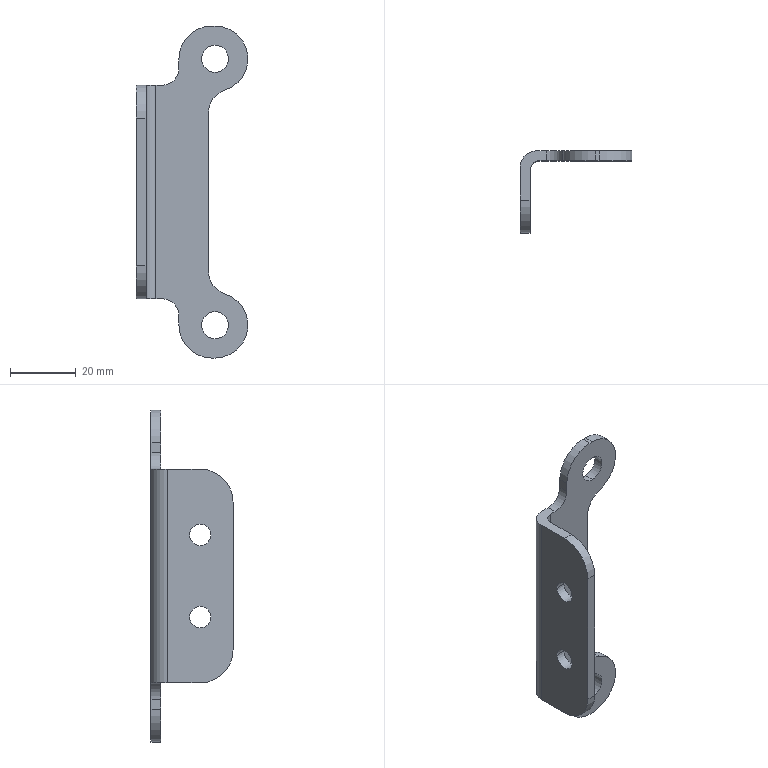Part | STEP file | IN-01-08-01-02-01 | 1 solid | 32 faces | box 34 x 25 x 101 mm | volume 9812 mm3 | cylinder 20 | plane 12 | commonest cylinder face diameters 20 x6 6.5 x4 8.2 x4 10 x3 14 x2 6 x1